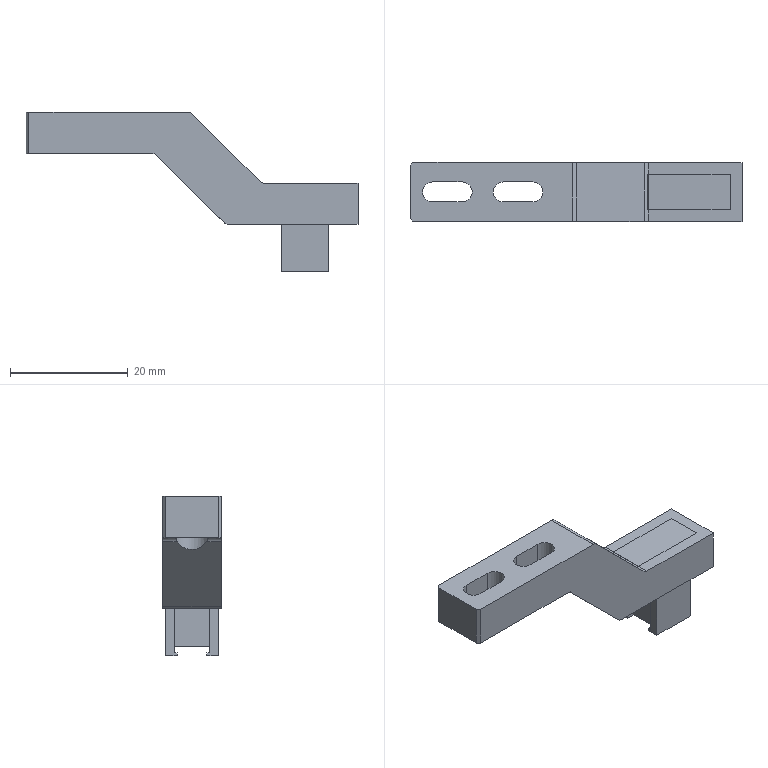NC program | NX | posted with a generic post | part box 56.3 x 10 x 27 mm
Lines 982 to 2462 of 3920, first 1366 of 1477 lines:
(ZLEVEL_PROFILE_COPY_2_COPY , TOOL : D4)
N1950 T04 M6
N1952 G54
N1954 G17 G0 G90 X-18.742 Y0.81 S9500 M3
N1956 G43 Z30. H4
N1958 Z-18.5
N1960 G94 G1 X-18.821 Y0.878 Z-18.505 F800.
N1962 X-19.178 Y1. Z-18.525
N1964 X-24.462 Z-18.802
N1966 X-24.792 Y0.893 Z-18.82
N1968 X-25.067 Y0.68 Z-18.839
N1970 X-25.253 Y0.387 Z-18.857
N1972 X-25.329 Y0.049 Z-18.875
N1974 X-25.286 Y-0.296 Z-18.893
N1976 X-25.166 Y-0.553 Z-18.908
N1978 X-24.977 Y-0.767 Z-18.923
N1980 X-24.736 Y-0.92 Z-18.938
N1982 X-24.462 Y-1. Z-18.953
N1984 X-19.178 Z-19.23
N1986 X-18.845 Y-0.891 Z-19.248
N1988 X-18.569 Y-0.675 Z-19.267
N1990 X-18.411 Y-0.439 Z-19.281
N1992 X-18.313 Y-0.074 Z-19.301
N1994 X-18.356 Y0.301 Z-19.321
N1996 X-18.534 Y0.634 Z-19.341
N1998 X-18.821 Y0.878 Z-19.361
N2000 X-19.178 Y1. Z-19.38
N2002 X-24.462 Z-19.657
N2004 X-24.792 Y0.893 Z-19.675
N2006 X-25.067 Y0.68 Z-19.694
N2008 X-25.253 Y0.387 Z-19.712
N2010 X-25.329 Y0.049 Z-19.73
N2012 X-25.286 Y-0.296 Z-19.748
N2014 X-25.166 Y-0.553 Z-19.763
N2016 X-24.977 Y-0.767 Z-19.778
N2018 X-24.736 Y-0.92 Z-19.793
N2020 X-24.462 Y-1. Z-19.808
N2022 X-19.178 Z-20.085
N2024 X-18.845 Y-0.891 Z-20.103
N2026 X-18.569 Y-0.675 Z-20.122
N2028 X-18.411 Y-0.439 Z-20.137
N2030 X-18.313 Y-0.074 Z-20.156
N2032 X-18.356 Y0.301 Z-20.176
N2034 X-18.534 Y0.634 Z-20.196
N2036 X-18.821 Y0.878 Z-20.216
N2038 X-19.178 Y1. Z-20.235
N2040 X-19.32 Z-20.243
N2042 X-24.32 F1100.
N2044 G3 X-25.32 Y0. R1.
N2046 X-24.32 Y-1. R1.
N2048 G1 X-19.32
N2050 G3 X-18.32 Y0. R1.
N2052 X-19.32 Y1. R1.
N2054 G1 X-19.459 Z-20.246
N2056 X-19.598 Y0.998 Z-20.248
N2058 X-19.737 Y1. Z-20.251
N2060 X-19.875 Y0.998 Z-20.254
N2062 X-20.014 Y1. Z-20.257
N2064 X-20.153 Y0.998 Z-20.259
N2066 X-20.292 Y1. Z-20.262
N2068 X-20.43 Y0.998 Z-20.265
N2070 X-20.569 Y1. Z-20.268
N2072 X-20.708 Y0.998 Z-20.27
N2074 X-20.847 Y1. Z-20.273
N2076 X-20.986 Y0.998 Z-20.276
N2078 X-21.124 Y1. Z-20.279
N2080 X-24.177 Z-20.339
N2082 X-24.316 Y0.994 Z-20.342
N2084 X-24.517 Y0.972 Z-20.346
N2086 X-24.588 Y0.955 Z-20.348
N2088 X-24.692 Y0.919 Z-20.35
N2090 X-24.776 Y0.883 Z-20.352
N2092 X-24.839 Y0.844 Z-20.353
N2094 X-24.987 Y0.733 Z-20.357
N2096 X-25.051 Y0.67 Z-20.359
N2098 X-25.152 Y0.539 Z-20.362
N2100 X-25.208 Y0.445 Z-20.364
N2102 X-25.248 Y0.349 Z-20.366
N2104 X-25.267 Y0.3 Z-20.367
N2106 X-25.276 Y0.261 Z-20.368
N2108 X-25.295 Y0.184 Z-20.37
N2110 X-25.308 Y0.079 Z-20.372
N2112 X-25.313 Y-0.013 Z-20.374
N2114 X-25.306 Y-0.089 Z-20.375
N2116 X-25.274 Y-0.267 Z-20.379
N2118 X-25.244 Y-0.356 Z-20.381
N2120 X-25.169 Y-0.51 Z-20.384
N2122 X-25.112 Y-0.597 Z-20.386
N2124 X-25.007 Y-0.716 Z-20.39
N2126 X-24.919 Y-0.791 Z-20.392
N2128 X-24.832 Y-0.848 Z-20.394
N2130 X-24.787 Y-0.875 Z-20.395
N2132 X-24.752 Y-0.893 Z-20.396
N2134 X-24.678 Y-0.923 Z-20.397
N2136 X-24.585 Y-0.954 Z-20.399
N2138 X-24.497 Y-0.975 Z-20.401
N2140 X-24.412 Y-0.985 Z-20.403
N2142 X-24.274 Y-1. Z-20.406
N2144 X-24.135 Z-20.408
N2146 X-20.249 Z-20.486
N2148 X-19.32
N2150 G3 X-18.32 Y0. R1.
N2152 X-19.32 Y1. R1.
N2154 G1 X-19.459 Z-20.488
N2156 X-19.598 Y0.998 Z-20.491
N2158 X-19.737 Y1. Z-20.494
N2160 X-19.875 Y0.998 Z-20.497
N2162 X-20.014 Y1. Z-20.5
N2164 X-20.153 Y0.998 Z-20.502
N2166 X-20.292 Y1. Z-20.505
N2168 X-20.43 Y0.998 Z-20.508
N2170 X-20.569 Y1. Z-20.511
N2172 X-20.708 Y0.998 Z-20.513
N2174 X-20.847 Y1. Z-20.516
N2176 X-20.986 Y0.998 Z-20.519
N2178 X-21.124 Y1. Z-20.522
N2180 X-24.177 Z-20.582
N2182 X-24.316 Y0.994 Z-20.585
N2184 X-24.517 Y0.972 Z-20.589
N2186 X-24.588 Y0.955 Z-20.591
N2188 X-24.692 Y0.919 Z-20.593
N2190 X-24.776 Y0.883 Z-20.595
N2192 X-24.839 Y0.844 Z-20.596
N2194 X-24.987 Y0.733 Z-20.6
N2196 X-25.051 Y0.67 Z-20.602
N2198 X-25.152 Y0.539 Z-20.605
N2200 X-25.208 Y0.445 Z-20.607
N2202 X-25.248 Y0.349 Z-20.609
N2204 X-25.267 Y0.3 Z-20.61
N2206 X-25.276 Y0.261 Z-20.611
N2208 X-25.294 Y0.184 Z-20.613
N2210 X-25.308 Y0.079 Z-20.615
N2212 X-25.313 Y-0.013 Z-20.617
N2214 X-25.306 Y-0.089 Z-20.618
N2216 X-25.274 Y-0.267 Z-20.622
N2218 X-25.244 Y-0.356 Z-20.624
N2220 X-25.169 Y-0.51 Z-20.627
N2222 X-25.112 Y-0.597 Z-20.629
N2224 X-25.007 Y-0.716 Z-20.632
N2226 X-24.919 Y-0.791 Z-20.635
N2228 X-24.832 Y-0.848 Z-20.637
N2230 X-24.787 Y-0.875 Z-20.638
N2232 X-24.752 Y-0.893 Z-20.639
N2234 X-24.678 Y-0.923 Z-20.64
N2236 X-24.585 Y-0.954 Z-20.642
N2238 X-24.497 Y-0.975 Z-20.644
N2240 X-24.412 Y-0.985 Z-20.646
N2242 X-24.274 Y-1. Z-20.649
N2244 X-24.135 Z-20.651
N2246 X-20.249 Z-20.729
N2248 X-19.32
N2250 G3 X-18.32 Y0. R1.
N2252 X-19.32 Y1. R1.
N2254 G1 X-19.459 Z-20.731
N2256 X-19.598 Y0.998 Z-20.734
N2258 X-19.737 Y1. Z-20.737
N2260 X-19.875 Y0.998 Z-20.74
N2262 X-20.014 Y1. Z-20.742
N2264 X-20.153 Y0.998 Z-20.745
N2266 X-20.292 Y1. Z-20.748
N2268 X-20.43 Y0.998 Z-20.751
N2270 X-20.569 Y1. Z-20.753
N2272 X-20.708 Y0.998 Z-20.756
N2274 X-20.847 Y1. Z-20.759
N2276 X-20.986 Y0.998 Z-20.762
N2278 X-21.124 Y1. Z-20.764
N2280 X-24.177 Z-20.825
N2282 X-24.316 Y0.994 Z-20.828
N2284 X-24.517 Y0.972 Z-20.832
N2286 X-24.588 Y0.955 Z-20.833
N2288 X-24.692 Y0.919 Z-20.836
N2290 X-24.776 Y0.883 Z-20.837
N2292 X-24.839 Y0.844 Z-20.839
N2294 X-24.986 Y0.733 Z-20.843
N2296 X-25.051 Y0.67 Z-20.844
N2298 X-25.151 Y0.54 Z-20.848
N2300 X-25.208 Y0.445 Z-20.85
N2302 X-25.248 Y0.349 Z-20.852
N2304 X-25.267 Y0.3 Z-20.853
N2306 X-25.276 Y0.262 Z-20.854
N2308 X-25.294 Y0.184 Z-20.856
N2310 X-25.308 Y0.079 Z-20.858
N2312 X-25.312 Y-0.013 Z-20.859
N2314 X-25.306 Y-0.089 Z-20.861
N2316 X-25.274 Y-0.266 Z-20.865
N2318 X-25.243 Y-0.356 Z-20.867
N2320 X-25.169 Y-0.51 Z-20.87
N2322 X-25.112 Y-0.597 Z-20.872
N2324 X-25.007 Y-0.716 Z-20.875
N2326 X-24.919 Y-0.791 Z-20.878
N2328 X-24.832 Y-0.848 Z-20.88
N2330 X-24.787 Y-0.875 Z-20.881
N2332 X-24.752 Y-0.892 Z-20.882
N2334 X-24.678 Y-0.923 Z-20.883
N2336 X-24.586 Y-0.954 Z-20.885
N2338 X-24.497 Y-0.975 Z-20.887
N2340 X-24.412 Y-0.985 Z-20.889
N2342 X-24.274 Y-1. Z-20.891
N2344 X-24.135 Z-20.894
N2346 X-20.249 Z-20.971
N2348 X-19.32
N2350 G3 X-18.32 Y0. R1.
N2352 X-19.32 Y1. R1.
N2354 G1 X-19.459 Z-20.974
N2356 X-19.598 Y0.998 Z-20.977
N2358 X-19.737 Y1. Z-20.98
N2360 X-19.875 Y0.998 Z-20.982
N2362 X-20.014 Y1. Z-20.985
N2364 X-20.153 Y0.998 Z-20.988
N2366 X-20.292 Y1. Z-20.991
N2368 X-20.43 Y0.998 Z-20.994
N2370 X-20.569 Y1. Z-20.996
N2372 X-20.708 Y0.998 Z-20.999
N2374 X-20.847 Y1. Z-21.002
N2376 X-20.986 Y0.998 Z-21.005
N2378 X-21.124 Y1. Z-21.007
N2380 X-24.177 Z-21.068
N2382 X-24.316 Y0.994 Z-21.071
N2384 X-24.517 Y0.972 Z-21.075
N2386 X-24.588 Y0.955 Z-21.076
N2388 X-24.692 Y0.919 Z-21.078
N2390 X-24.776 Y0.882 Z-21.08
N2392 X-24.839 Y0.844 Z-21.082
N2394 X-24.986 Y0.733 Z-21.086
N2396 X-25.051 Y0.67 Z-21.087
N2398 X-25.151 Y0.54 Z-21.091
N2400 X-25.208 Y0.445 Z-21.093
N2402 X-25.248 Y0.349 Z-21.095
N2404 X-25.266 Y0.3 Z-21.096
N2406 X-25.294 Y0.184 Z-21.098
N2408 X-25.308 Y0.079 Z-21.101
N2410 X-25.312 Y-0.012 Z-21.102
N2412 X-25.306 Y-0.089 Z-21.104
N2414 X-25.274 Y-0.266 Z-21.108
N2416 X-25.243 Y-0.356 Z-21.109
N2418 X-25.169 Y-0.509 Z-21.113
N2420 X-25.112 Y-0.597 Z-21.115
N2422 X-25.007 Y-0.715 Z-21.118
N2424 X-24.919 Y-0.791 Z-21.12
N2426 X-24.832 Y-0.848 Z-21.123
N2428 X-24.787 Y-0.874 Z-21.124
N2430 X-24.752 Y-0.892
N2432 X-24.678 Y-0.922 Z-21.126
N2434 X-24.586 Y-0.954 Z-21.128
N2436 X-24.497 Y-0.975 Z-21.13
N2438 X-24.412 Y-0.985 Z-21.131
N2440 X-24.274 Y-1. Z-21.134
N2442 X-24.135 Z-21.137
N2444 X-20.249 Z-21.214
N2446 X-19.32
N2448 G3 X-18.32 Y0. R1.
N2450 X-19.32 Y1. R1.
N2452 G1 X-19.459 Z-21.217
N2454 X-19.598 Y0.998 Z-21.22
N2456 X-19.737 Y1. Z-21.223
N2458 X-19.875 Y0.998 Z-21.225
N2460 X-20.014 Y1. Z-21.228
N2462 X-20.153 Y0.998 Z-21.231
N2464 X-20.292 Y1. Z-21.234
N2466 X-20.43 Y0.998 Z-21.236
N2468 X-20.569 Y1. Z-21.239
N2470 X-20.708 Y0.998 Z-21.242
N2472 X-20.847 Y1. Z-21.245
N2474 X-20.986 Y0.998 Z-21.247
N2476 X-21.124 Y1. Z-21.25
N2478 X-24.177 Z-21.311
N2480 X-24.316 Y0.994 Z-21.314
N2482 X-24.518 Y0.971 Z-21.318
N2484 X-24.588 Y0.955 Z-21.319
N2486 X-24.692 Y0.919 Z-21.321
N2488 X-24.776 Y0.882 Z-21.323
N2490 X-24.839 Y0.844 Z-21.325
N2492 X-24.986 Y0.733 Z-21.328
N2494 X-25.051 Y0.67 Z-21.33
N2496 X-25.151 Y0.54 Z-21.333
N2498 X-25.208 Y0.445 Z-21.336
N2500 X-25.248 Y0.349 Z-21.338
N2502 X-25.266 Y0.3 Z-21.339
N2504 X-25.294 Y0.184 Z-21.341
N2506 X-25.308 Y0.079 Z-21.343
N2508 X-25.312 Y-0.012 Z-21.345
N2510 X-25.306 Y-0.089 Z-21.347
N2512 X-25.274 Y-0.266 Z-21.35
N2514 X-25.243 Y-0.356 Z-21.352
N2516 X-25.169 Y-0.509 Z-21.356
N2518 X-25.112 Y-0.597 Z-21.358
N2520 X-25.007 Y-0.715 Z-21.361
N2522 X-24.919 Y-0.791 Z-21.363
N2524 X-24.832 Y-0.848 Z-21.365
N2526 X-24.787 Y-0.874 Z-21.366
N2528 X-24.752 Y-0.892 Z-21.367
N2530 X-24.678 Y-0.922 Z-21.369
N2532 X-24.586 Y-0.953 Z-21.371
N2534 X-24.497 Y-0.975 Z-21.373
N2536 X-24.412 Y-0.985 Z-21.374
N2538 X-24.274 Y-1. Z-21.377
N2540 X-24.135 Z-21.38
N2542 X-20.249 Z-21.457
N2544 X-19.32
N2546 G3 X-18.32 Y0. R1.
N2548 X-19.32 Y1. R1.
N2550 G1 X-19.459 Z-21.46
N2552 X-19.598 Y0.998 Z-21.463
N2554 X-19.737 Y1. Z-21.465
N2556 X-19.875 Y0.998 Z-21.468
N2558 X-20.014 Y1. Z-21.471
N2560 X-20.153 Y0.998 Z-21.474
N2562 X-20.292 Y1. Z-21.476
N2564 X-20.43 Y0.998 Z-21.479
N2566 X-20.569 Y1. Z-21.482
N2568 X-20.708 Y0.998 Z-21.485
N2570 X-20.847 Y1. Z-21.488
N2572 X-20.986 Y0.998 Z-21.49
N2574 X-21.124 Y1. Z-21.493
N2576 X-24.177 Z-21.554
N2578 X-24.316 Y0.994 Z-21.556
N2580 X-24.518 Y0.971 Z-21.561
N2582 X-24.588 Y0.955 Z-21.562
N2584 X-24.691 Y0.919 Z-21.564
N2586 X-24.775 Y0.882 Z-21.566
N2588 X-24.839 Y0.844 Z-21.568
N2590 X-24.986 Y0.733 Z-21.571
N2592 X-25.051 Y0.67 Z-21.573
N2594 X-25.151 Y0.54 Z-21.576
N2596 X-25.208 Y0.445 Z-21.579
N2598 X-25.248 Y0.349 Z-21.581
N2600 X-25.266 Y0.3 Z-21.582
N2602 X-25.294 Y0.184 Z-21.584
N2604 X-25.308 Y0.079 Z-21.586
N2606 X-25.312 Y-0.012 Z-21.588
N2608 X-25.306 Y-0.089 Z-21.59
N2610 X-25.274 Y-0.266 Z-21.593
N2612 X-25.243 Y-0.356 Z-21.595
N2614 X-25.169 Y-0.509 Z-21.599
N2616 X-25.112 Y-0.597 Z-21.601
N2618 X-25.007 Y-0.715 Z-21.604
N2620 X-24.918 Y-0.791 Z-21.606
N2622 X-24.832 Y-0.847 Z-21.608
N2624 X-24.787 Y-0.874 Z-21.609
N2626 X-24.752 Y-0.892 Z-21.61
N2628 X-24.678 Y-0.922 Z-21.612
N2630 X-24.586 Y-0.953 Z-21.614
N2632 X-24.497 Y-0.975 Z-21.615
N2634 X-24.412 Y-0.985 Z-21.617
N2636 X-24.274 Y-1. Z-21.62
N2638 X-24.135 Z-21.623
N2640 X-20.249 Z-21.7
N2642 X-19.32
N2644 G3 X-18.32 Y0. R1.
N2646 X-19.32 Y1. R1.
N2648 G1 X-19.459 Z-21.703
N2650 X-19.598 Y0.998 Z-21.706
N2652 X-19.737 Y1. Z-21.708
N2654 X-19.875 Y0.998 Z-21.711
N2656 X-20.014 Y1. Z-21.714
N2658 X-20.153 Y0.998 Z-21.717
N2660 X-20.292 Y1. Z-21.719
N2662 X-20.43 Y0.998 Z-21.722
N2664 X-20.569 Y1. Z-21.725
N2666 X-20.708 Y0.998 Z-21.728
N2668 X-20.847 Y1. Z-21.73
N2670 X-20.986 Y0.998 Z-21.733
N2672 X-21.124 Y1. Z-21.736
N2674 X-24.177 Z-21.797
N2676 X-24.316 Y0.994 Z-21.799
N2678 X-24.518 Y0.971 Z-21.803
N2680 X-24.588 Y0.955 Z-21.805
N2682 X-24.691 Y0.919 Z-21.807
N2684 X-24.775 Y0.882 Z-21.809
N2686 X-24.839 Y0.844 Z-21.81
N2688 X-24.986 Y0.734 Z-21.814
N2690 X-25.051 Y0.67 Z-21.816
N2692 X-25.153 Y0.537 Z-21.819
N2694 X-25.208 Y0.445 Z-21.821
N2696 X-25.248 Y0.348 Z-21.824
N2698 X-25.266 Y0.3 Z-21.825
N2700 X-25.294 Y0.184 Z-21.827
N2702 X-25.308 Y0.079 Z-21.829
N2704 X-25.313 Y-0.012 Z-21.831
N2706 X-25.306 Y-0.089 Z-21.832
N2708 X-25.272 Y-0.272 Z-21.836
N2710 X-25.243 Y-0.356 Z-21.838
N2712 X-25.168 Y-0.511 Z-21.841
N2714 X-25.112 Y-0.597 Z-21.844
N2716 X-25.007 Y-0.715 Z-21.847
N2718 X-24.918 Y-0.791 Z-21.849
N2720 X-24.832 Y-0.847 Z-21.851
N2722 X-24.787 Y-0.874 Z-21.852
N2724 X-24.752 Y-0.892 Z-21.853
N2726 X-24.678 Y-0.922 Z-21.855
N2728 X-24.586 Y-0.953 Z-21.856
N2730 X-24.497 Y-0.975 Z-21.858
N2732 X-24.412 Y-0.985 Z-21.86
N2734 X-24.274 Y-1. Z-21.863
N2736 X-24.135 Z-21.866
N2738 X-20.249 Z-21.943
N2740 X-19.32
N2742 G3 X-18.32 Y0. R1.
N2744 X-19.32 Y1. R1.
N2746 G1 X-19.459 Z-21.946
N2748 X-19.598 Y0.998 Z-21.948
N2750 X-19.737 Y1. Z-21.951
N2752 X-19.875 Y0.998 Z-21.954
N2754 X-20.014 Y1. Z-21.957
N2756 X-20.153 Y0.998 Z-21.959
N2758 X-20.292 Y1. Z-21.962
N2760 X-20.43 Y0.998 Z-21.965
N2762 X-20.569 Y1. Z-21.968
N2764 X-20.708 Y0.998 Z-21.97
N2766 X-20.847 Y1. Z-21.973
N2768 X-20.986 Y0.998 Z-21.976
N2770 X-21.124 Y1. Z-21.979
N2772 X-24.177 Z-22.039
N2774 X-24.316 Y0.994 Z-22.042
N2776 X-24.518 Y0.971 Z-22.046
N2778 X-24.588 Y0.954 Z-22.048
N2780 X-24.691 Y0.919 Z-22.05
N2782 X-24.775 Y0.882 Z-22.052
N2784 X-24.839 Y0.844 Z-22.053
N2786 X-24.986 Y0.734 Z-22.057
N2788 X-25.051 Y0.67 Z-22.059
N2790 X-25.153 Y0.537 Z-22.062
N2792 X-25.207 Y0.445 Z-22.064
N2794 X-25.248 Y0.348 Z-22.066
N2796 X-25.266 Y0.3 Z-22.067
N2798 X-25.294 Y0.184 Z-22.07
N2800 X-25.307 Y0.079 Z-22.072
N2802 X-25.313 Y-0.012 Z-22.074
N2804 X-25.306 Y-0.089 Z-22.075
N2806 X-25.272 Y-0.271 Z-22.079
N2808 X-25.243 Y-0.356 Z-22.081
N2810 X-25.168 Y-0.511 Z-22.084
N2812 X-25.112 Y-0.597 Z-22.086
N2814 X-25.007 Y-0.715 Z-22.09
N2816 X-24.918 Y-0.791 Z-22.092
N2818 X-24.832 Y-0.847 Z-22.094
N2820 X-24.787 Y-0.874 Z-22.095
N2822 X-24.752 Y-0.892 Z-22.096
N2824 X-24.678 Y-0.922 Z-22.097
N2826 X-24.587 Y-0.954 Z-22.099
N2828 X-24.498 Y-0.975 Z-22.101
N2830 X-24.412 Y-0.985 Z-22.103
N2832 X-24.274 Y-1. Z-22.106
N2834 X-24.135 Z-22.108
N2836 X-20.249 Z-22.186
N2838 X-19.32
N2840 G3 X-18.32 Y0. R1.
N2842 X-19.32 Y1. R1.
N2844 G1 X-19.459 Z-22.188
N2846 X-19.598 Y0.998 Z-22.191
N2848 X-19.737 Y1. Z-22.194
N2850 X-19.875 Y0.998 Z-22.197
N2852 X-20.014 Y1. Z-22.2
N2854 X-20.153 Y0.998 Z-22.202
N2856 X-20.292 Y1. Z-22.205
N2858 X-20.43 Y0.998 Z-22.208
N2860 X-20.569 Y1. Z-22.211
N2862 X-20.708 Y0.998 Z-22.213
N2864 X-20.847 Y1. Z-22.216
N2866 X-20.986 Y0.998 Z-22.219
N2868 X-21.124 Y1. Z-22.222
N2870 X-24.177 Z-22.282
N2872 X-24.316 Y0.994 Z-22.285
N2874 X-24.518 Y0.971 Z-22.289
N2876 X-24.588 Y0.954 Z-22.291
N2878 X-24.691 Y0.919 Z-22.293
N2880 X-24.775 Y0.882 Z-22.295
N2882 X-24.839 Y0.844 Z-22.296
N2884 X-24.986 Y0.735 Z-22.3
N2886 X-25.051 Y0.67 Z-22.302
N2888 X-25.153 Y0.537 Z-22.305
N2890 X-25.207 Y0.445 Z-22.307
N2892 X-25.248 Y0.349 Z-22.309
N2894 X-25.266 Y0.3 Z-22.31
N2896 X-25.294 Y0.184 Z-22.313
N2898 X-25.307 Y0.079 Z-22.315
N2900 X-25.313 Y-0.012 Z-22.317
N2902 X-25.306 Y-0.089 Z-22.318
N2904 X-25.272 Y-0.271 Z-22.322
N2906 X-25.243 Y-0.356 Z-22.324
N2908 X-25.168 Y-0.51 Z-22.327
N2910 X-25.112 Y-0.597 Z-22.329
N2912 X-25.007 Y-0.715 Z-22.332
N2914 X-24.918 Y-0.791 Z-22.335
N2916 X-24.832 Y-0.847 Z-22.337
N2918 X-24.788 Y-0.874 Z-22.338
N2920 X-24.752 Y-0.892 Z-22.339
N2922 X-24.678 Y-0.922 Z-22.34
N2924 X-24.587 Y-0.954 Z-22.342
N2926 X-24.498 Y-0.975 Z-22.344
N2928 X-24.412 Y-0.985 Z-22.346
N2930 X-24.274 Y-1. Z-22.349
N2932 X-24.135 Z-22.351
N2934 X-20.249 Z-22.429
N2936 X-19.32
N2938 G3 X-18.32 Y0. R1.
N2940 X-19.32 Y1. R1.
N2942 G1 X-19.459 Z-22.431
N2944 X-19.598 Y0.998 Z-22.434
N2946 X-19.737 Y1. Z-22.437
N2948 X-19.875 Y0.998 Z-22.44
N2950 X-20.014 Y1. Z-22.442
N2952 X-20.153 Y0.998 Z-22.445
N2954 X-20.292 Y1. Z-22.448
N2956 X-20.43 Y0.998 Z-22.451
N2958 X-20.569 Y1. Z-22.453
N2960 X-20.708 Y0.998 Z-22.456
N2962 X-20.847 Y1. Z-22.459
N2964 X-20.986 Y0.998 Z-22.462
N2966 X-21.124 Y1. Z-22.464
N2968 X-24.177 Z-22.525
N2970 X-24.316 Y0.994 Z-22.528
N2972 X-24.518 Y0.971 Z-22.532
N2974 X-24.588 Y0.954 Z-22.533
N2976 X-24.691 Y0.918 Z-22.536
N2978 X-24.775 Y0.882 Z-22.537
N2980 X-24.839 Y0.844 Z-22.539
N2982 X-24.986 Y0.735 Z-22.543
N2984 X-25.051 Y0.67 Z-22.544
N2986 X-25.153 Y0.537 Z-22.548
N2988 X-25.207 Y0.445 Z-22.55
N2990 X-25.248 Y0.349 Z-22.552
N2992 X-25.267 Y0.3 Z-22.553
N2994 X-25.294 Y0.184 Z-22.556
N2996 X-25.307 Y0.077 Z-22.558
N2998 X-25.312 Y-0.014 Z-22.56
N3000 X-25.305 Y-0.089 Z-22.561
N3002 X-25.273 Y-0.266 Z-22.565
N3004 X-25.243 Y-0.356 Z-22.567
N3006 X-25.169 Y-0.509 Z-22.57
N3008 X-25.112 Y-0.597 Z-22.572
N3010 X-25.007 Y-0.715 Z-22.575
N3012 X-24.918 Y-0.791 Z-22.578
N3014 X-24.832 Y-0.847 Z-22.58
N3016 X-24.788 Y-0.874 Z-22.581
N3018 X-24.752 Y-0.892 Z-22.582
N3020 X-24.678 Y-0.922 Z-22.583
N3022 X-24.587 Y-0.954 Z-22.585
N3024 X-24.498 Y-0.975 Z-22.587
N3026 X-24.412 Y-0.985 Z-22.589
N3028 X-24.274 Y-1. Z-22.591
N3030 X-24.135 Z-22.594
N3032 X-20.249 Z-22.671
N3034 X-19.32
N3036 G3 X-18.32 Y0. R1.
N3038 X-19.32 Y1. R1.
N3040 G1 X-19.459 Z-22.674
N3042 X-19.598 Y0.998 Z-22.677
N3044 X-19.737 Y1. Z-22.68
N3046 X-19.875 Y0.998 Z-22.682
N3048 X-20.014 Y1. Z-22.685
N3050 X-20.153 Y0.998 Z-22.688
N3052 X-20.292 Y1. Z-22.691
N3054 X-20.43 Y0.998 Z-22.694
N3056 X-20.569 Y1. Z-22.696
N3058 X-20.708 Y0.998 Z-22.699
N3060 X-20.847 Y1. Z-22.702
N3062 X-20.986 Y0.998 Z-22.705
N3064 X-21.124 Y1. Z-22.707
N3066 X-24.177 Z-22.768
N3068 X-24.316 Y0.993 Z-22.771
N3070 X-24.518 Y0.971 Z-22.775
N3072 X-24.588 Y0.954 Z-22.776
N3074 X-24.691 Y0.918 Z-22.778
N3076 X-24.775 Y0.882 Z-22.78
N3078 X-24.839 Y0.844 Z-22.782
N3080 X-24.985 Y0.735 Z-22.785
N3082 X-25.051 Y0.67 Z-22.787
N3084 X-25.152 Y0.537 Z-22.791
N3086 X-25.207 Y0.445 Z-22.793
N3088 X-25.248 Y0.349 Z-22.795
N3090 X-25.267 Y0.3 Z-22.796
N3092 X-25.276 Y0.262 Z-22.797
N3094 X-25.294 Y0.184 Z-22.798
N3096 X-25.307 Y0.076 Z-22.801
N3098 X-25.312 Y-0.015 Z-22.802
N3100 X-25.305 Y-0.089 Z-22.804
N3102 X-25.273 Y-0.267 Z-22.808
N3104 X-25.243 Y-0.356 Z-22.809
N3106 X-25.169 Y-0.509 Z-22.813
N3108 X-25.112 Y-0.597 Z-22.815
N3110 X-25.007 Y-0.715 Z-22.818
N3112 X-24.918 Y-0.791 Z-22.82
N3114 X-24.832 Y-0.847 Z-22.823
N3116 X-24.788 Y-0.874 Z-22.824
N3118 X-24.752 Y-0.892
N3120 X-24.678 Y-0.922 Z-22.826
N3122 X-24.587 Y-0.954 Z-22.828
N3124 X-24.498 Y-0.974 Z-22.83
N3126 X-24.412 Y-0.985 Z-22.831
N3128 X-24.274 Y-1. Z-22.834
N3130 X-24.135 Z-22.837
N3132 X-20.249 Z-22.914
N3134 X-19.32
N3136 G3 X-18.32 Y0. R1.
N3138 X-19.32 Y1. R1.
N3140 G1 X-24.233 Z-23.012
N3142 X-24.374 Y0.999 Z-23.015
N3144 X-24.513 Y0.981 Z-23.018
N3146 X-24.648 Y0.945 Z-23.02
N3148 X-24.777 Y0.89 Z-23.023
N3150 X-24.897 Y0.817 Z-23.026
N3152 X-25.006 Y0.728 Z-23.029
N3154 X-25.101 Y0.625 Z-23.032
N3156 X-25.181 Y0.51 Z-23.034
N3158 X-25.243 Y0.384 Z-23.037
N3160 X-25.288 Y0.251 Z-23.04
N3162 X-25.314 Y0.113 Z-23.043
N3164 X-25.32 Y-0.027 Z-23.045
N3166 X-25.306 Y-0.166 Z-23.048
N3168 X-25.273 Y-0.303 Z-23.051
N3170 X-25.222 Y-0.433 Z-23.054
N3172 X-25.152 Y-0.555 Z-23.057
N3174 X-25.066 Y-0.666 Z-23.059
N3176 X-24.966 Y-0.764 Z-23.062
N3178 X-24.853 Y-0.846 Z-23.065
N3180 X-24.729 Y-0.913 Z-23.068
N3182 X-24.597 Y-0.961 Z-23.071
N3184 X-24.46 Y-0.99 Z-23.073
N3186 X-24.32 Y-1. Z-23.076
N3188 X-20.249 Z-23.157
N3190 X-19.32
N3192 G3 X-18.32 Y0. R1.
N3194 X-19.32 Y1. R1.
N3196 G1 X-24.233 Z-23.255
N3198 X-24.374 Y0.999 Z-23.258
N3200 X-24.513 Y0.981 Z-23.26
N3202 X-24.648 Y0.945 Z-23.263
N3204 X-24.777 Y0.89 Z-23.266
N3206 X-24.897 Y0.817 Z-23.269
N3208 X-25.006 Y0.728 Z-23.272
N3210 X-25.101 Y0.625 Z-23.274
N3212 X-25.181 Y0.51 Z-23.277
N3214 X-25.243 Y0.384 Z-23.28
N3216 X-25.288 Y0.251 Z-23.283
N3218 X-25.314 Y0.113 Z-23.286
N3220 X-25.32 Y-0.027 Z-23.288
N3222 X-25.306 Y-0.166 Z-23.291
N3224 X-25.273 Y-0.303 Z-23.294
N3226 X-25.222 Y-0.433 Z-23.297
N3228 X-25.152 Y-0.555 Z-23.3
N3230 X-25.066 Y-0.666 Z-23.302
N3232 X-24.966 Y-0.764 Z-23.305
N3234 X-24.853 Y-0.846 Z-23.308
N3236 X-24.729 Y-0.913 Z-23.311
N3238 X-24.597 Y-0.961 Z-23.313
N3240 X-24.46 Y-0.99 Z-23.316
N3242 X-24.32 Y-1. Z-23.319
N3244 X-20.249 Z-23.4
N3246 X-19.32
N3248 G3 X-18.32 Y0. R1.
N3250 X-19.32 Y1. R1.
N3252 G1 X-24.32
N3254 G3 X-25.32 Y0. R1.
N3256 X-24.32 Y-1. R1.
N3258 G1 X-20.249
N3260 Z-21.9
N3262 G0 Z30.
N3264 X-6.378 Y0.342
N3266 Z-18.5
N3268 G1 X-6.393 Y0.4 Z-18.503 F800.
N3270 X-6.562 Y0.667 Z-18.52
N3272 X-6.669 Y0.759 Z-18.527
N3274 X-6.688 Y0.746 Z-18.528
N3276 X-7.155 Y0.891 Z-18.554
N3278 X-7.406 Y1. Z-18.568
N3280 X-12.462 Z-18.833
N3282 X-12.792 Y0.893 Z-18.851
N3284 X-13.067 Y0.68 Z-18.87
N3286 X-13.253 Y0.387 Z-18.888
N3288 X-13.329 Y0.048 Z-18.906
N3290 X-13.286 Y-0.296 Z-18.924
N3292 X-13.166 Y-0.553 Z-18.939
N3294 X-12.977 Y-0.767 Z-18.954
N3296 X-12.736 Y-0.92 Z-18.969
N3298 X-12.462 Y-1. Z-18.984
N3300 X-7.178 Z-19.261
N3302 X-6.806 Y-0.87 Z-19.282
N3304 X-6.513 Y-0.607 Z-19.302
N3306 X-6.444 Y-0.482 Z-19.31
N3308 X-6.467 Y-0.464 Z-19.311
N3310 X-6.463 Y-0.434 Z-19.313
N3312 X-6.437 Y-0.422 Z-19.314
N3314 X-6.443 Y-0.386 Z-19.316
N3316 X-6.42 Y-0.356 Z-19.318
N3318 X-6.384 Y-0.353 Z-19.32
N3320 X-6.334 Y-0.22 Z-19.327
N3322 X-6.315 Y0.095 Z-19.344
N3324 X-6.393 Y0.4 Z-19.36
N3326 X-6.562 Y0.667 Z-19.377
N3328 X-6.669 Y0.759 Z-19.384
N3330 X-6.688 Y0.746 Z-19.386
N3332 X-7.155 Y0.891 Z-19.411
N3334 X-7.406 Y1. Z-19.426
N3336 X-12.462 Z-19.691
N3338 X-12.792 Y0.893 Z-19.709
N3340 X-13.067 Y0.68 Z-19.727
N3342 X-13.253 Y0.387 Z-19.745
N3344 X-13.329 Y0.048 Z-19.763
N3346 X-13.286 Y-0.296 Z-19.781
N3348 X-13.166 Y-0.553 Z-19.796
N3350 X-12.977 Y-0.767 Z-19.811
N3352 X-12.736 Y-0.92 Z-19.826
N3354 X-12.462 Y-1. Z-19.841
N3356 X-7.178 Z-20.118
N3358 X-6.806 Y-0.87 Z-20.139
N3360 X-6.513 Y-0.607 Z-20.159
N3362 X-6.444 Y-0.482 Z-20.167
N3364 X-6.467 Y-0.464 Z-20.168
N3366 X-6.463 Y-0.434 Z-20.17
N3368 X-6.437 Y-0.422 Z-20.171
N3370 X-6.443 Y-0.386 Z-20.173
N3372 X-6.42 Y-0.356 Z-20.175
N3374 X-6.384 Y-0.353 Z-20.177
N3376 X-6.334 Y-0.22 Z-20.185
N3378 X-6.315 Y0.095 Z-20.201
N3380 X-6.393 Y0.4 Z-20.218
N3382 X-6.562 Y0.667 Z-20.234
N3384 X-6.669 Y0.759 Z-20.242
N3386 X-6.688 Y0.746 Z-20.243
N3388 X-7.155 Y0.891 F1100.
N3390 X-7.406 Y1.
N3392 X-12.32
N3394 G3 X-13.32 Y0. R1.
N3396 X-12.32 Y-1. R1.
N3398 G1 X-7.32
N3400 G3 X-6.444 Y-0.482 R1.
N3402 G1 X-6.467 Y-0.464
N3404 X-6.463 Y-0.434
N3406 X-6.437 Y-0.422
N3408 X-6.443 Y-0.386
N3410 X-6.42 Y-0.356
N3412 X-6.384 Y-0.353
N3414 G3 X-6.669 Y0.759 R1.
N3416 G1 X-6.688 Y0.746
N3418 X-6.821 Y0.788 Z-20.246
N3420 X-6.953 Y0.829 Z-20.248
N3422 X-7.086 Y0.87 Z-20.251
N3424 X-7.218 Y0.914 Z-20.254
N3426 X-7.282 Y0.939 Z-20.255
N3428 X-7.345 Y0.967 Z-20.257
N3430 X-7.377 Y0.981
N3432 X-7.408 Y0.996 Z-20.258
N3434 X-7.443 Y0.998 Z-20.259
N3436 X-7.477
N3438 X-7.616 Y1. Z-20.262
N3440 X-7.755 Y0.999 Z-20.265
N3442 X-7.894 Y0.998 Z-20.268
N3444 X-8.033 Z-20.27
N3446 X-8.172 Z-20.273
N3448 X-8.311 Z-20.276
N3450 X-8.449 Z-20.279
N3452 X-8.588 Z-20.281
N3454 X-8.727 Z-20.284
N3456 X-8.866 Z-20.287
N3458 X-9.005 Y1. Z-20.29
N3460 X-12.201 Z-20.353
N3462 X-12.339 Y0.992 Z-20.356
N3464 X-12.477 Y0.981 Z-20.359
N3466 X-12.574 Y0.958 Z-20.361
N3468 X-12.623 Y0.946 Z-20.362
N3470 X-12.662 Y0.93 Z-20.363
N3472 X-12.739 Y0.899 Z-20.364
N3474 X-12.834 Y0.848 Z-20.366
N3476 X-12.911 Y0.799 Z-20.368
N3478 X-12.969 Y0.749 Z-20.37
N3480 X-13.096 Y0.617 Z-20.373
N3482 X-13.15 Y0.543 Z-20.375
N3484 X-13.23 Y0.393 Z-20.379
N3486 X-13.268 Y0.295 Z-20.381
N3488 X-13.292 Y0.194 Z-20.383
N3490 X-13.302 Y0.143 Z-20.384
N3492 X-13.306 Y0.103 Z-20.385
N3494 X-13.311 Y0.023 Z-20.386
N3496 X-13.307 Y-0.088 Z-20.389
N3498 X-13.302 Y-0.144 Z-20.39
N3500 X-13.295 Y-0.179
N3502 X-13.278 Y-0.249 Z-20.392
N3504 X-13.218 Y-0.417 Z-20.395
N3506 X-13.173 Y-0.502 Z-20.397
N3508 X-13.076 Y-0.638 Z-20.401
N3510 X-13.003 Y-0.718 Z-20.403
N3512 X-12.878 Y-0.819 Z-20.406
N3514 X-12.781 Y-0.878 Z-20.408
N3516 X-12.647 Y-0.936 Z-20.411
N3518 X-12.522 Y-0.97 Z-20.414
N3520 X-12.385 Y-0.988 Z-20.417
N3522 X-12.247 Y-1. Z-20.419
N3524 X-8.913 Z-20.486
N3526 X-7.32
N3528 G3 X-6.444 Y-0.482 R1.
N3530 G1 X-6.467 Y-0.464
N3532 X-6.463 Y-0.434
N3534 X-6.437 Y-0.422
N3536 X-6.443 Y-0.386
N3538 X-6.42 Y-0.356
N3540 X-6.384 Y-0.353
N3542 G3 X-6.669 Y0.759 R1.
N3544 G1 X-6.688 Y0.746
N3546 X-6.821 Y0.788 Z-20.488
N3548 X-6.953 Y0.829 Z-20.491
N3550 X-7.086 Y0.87 Z-20.494
N3552 X-7.218 Y0.914 Z-20.497
N3554 X-7.282 Y0.939 Z-20.498
N3556 X-7.345 Y0.967 Z-20.5
N3558 X-7.377 Y0.982
N3560 X-7.408 Y0.995 Z-20.501
N3562 X-7.443 Y0.998 Z-20.502
N3564 X-7.477
N3566 X-7.616 Y1. Z-20.505
N3568 X-7.755 Y0.999 Z-20.508
N3570 X-7.894 Y0.998 Z-20.511
N3572 X-8.033 Z-20.513
N3574 X-8.172 Z-20.516
N3576 X-8.311 Z-20.519
N3578 X-8.449 Z-20.522
N3580 X-8.588 Z-20.524
N3582 X-8.727 Z-20.527
N3584 X-8.866 Z-20.53
N3586 X-9.005 Y1. Z-20.533
N3588 X-12.201 Z-20.596
N3590 X-12.339 Y0.992 Z-20.599
N3592 X-12.477 Y0.981 Z-20.602
N3594 X-12.574 Y0.958 Z-20.604
N3596 X-12.623 Y0.946 Z-20.605
N3598 X-12.662 Y0.93
N3600 X-12.739 Y0.899 Z-20.607
N3602 X-12.833 Y0.848 Z-20.609
N3604 X-12.911 Y0.799 Z-20.611
N3606 X-12.969 Y0.749 Z-20.613
N3608 X-13.096 Y0.617 Z-20.616
N3610 X-13.15 Y0.543 Z-20.618
N3612 X-13.23 Y0.393 Z-20.622
N3614 X-13.268 Y0.295 Z-20.624
N3616 X-13.292 Y0.194 Z-20.626
N3618 X-13.302 Y0.144 Z-20.627
N3620 X-13.306 Y0.104 Z-20.628
N3622 X-13.311 Y0.023 Z-20.629
N3624 X-13.307 Y-0.088 Z-20.631
N3626 X-13.302 Y-0.144 Z-20.633
N3628 X-13.295 Y-0.179
N3630 X-13.278 Y-0.249 Z-20.635
N3632 X-13.218 Y-0.417 Z-20.638
N3634 X-13.173 Y-0.502 Z-20.64
N3636 X-13.076 Y-0.638 Z-20.644
N3638 X-13.003 Y-0.718 Z-20.646
N3640 X-12.878 Y-0.819 Z-20.649
N3642 X-12.781 Y-0.878 Z-20.651
N3644 X-12.647 Y-0.936 Z-20.654
N3646 X-12.522 Y-0.97 Z-20.657
N3648 X-12.385 Y-0.988 Z-20.66
N3650 X-12.247 Y-1. Z-20.662
N3652 X-8.913 Z-20.729
N3654 X-7.32
N3656 G3 X-6.444 Y-0.482 R1.
N3658 G1 X-6.467 Y-0.464
N3660 X-6.463 Y-0.434
N3662 X-6.437 Y-0.422
N3664 X-6.443 Y-0.386
N3666 X-6.42 Y-0.356
N3668 X-6.384 Y-0.353
N3670 G3 X-6.669 Y0.759 R1.
N3672 G1 X-6.688 Y0.746
N3674 X-6.821 Y0.788 Z-20.731
N3676 X-6.953 Y0.829 Z-20.734
N3678 X-7.086 Y0.87 Z-20.737
N3680 X-7.218 Y0.914 Z-20.74
N3682 X-7.282 Y0.939 Z-20.741
N3684 X-7.345 Y0.967 Z-20.742
N3686 X-7.377 Y0.981 Z-20.743
N3688 X-7.408 Y0.996 Z-20.744
N3690 X-7.443 Y0.997
N3692 X-7.477 Y0.998 Z-20.745
N3694 X-7.616 Y1. Z-20.748
N3696 X-7.755 Y0.998 Z-20.751
N3698 X-7.894 Z-20.753
N3700 X-8.033 Z-20.756
N3702 X-8.172 Z-20.759
N3704 X-8.311 Z-20.762
N3706 X-8.449 Z-20.764
N3708 X-8.588 Z-20.767
N3710 X-8.727 Z-20.77
N3712 X-8.866 Z-20.773
N3714 X-9.005 Y1. Z-20.775
N3716 X-12.201 Z-20.839
N3718 X-12.339 Y0.992 Z-20.842
N3720 X-12.477 Y0.981 Z-20.844
N3722 X-12.574 Y0.958 Z-20.846
N3724 X-12.623 Y0.946 Z-20.847
N3726 X-12.662 Y0.93 Z-20.848
N3728 X-12.739 Y0.899 Z-20.85
N3730 X-12.833 Y0.848 Z-20.852
N3732 X-12.91 Y0.799 Z-20.854
N3734 X-12.969 Y0.749 Z-20.856
N3736 X-13.096 Y0.617 Z-20.859
N3738 X-13.15 Y0.543 Z-20.861
N3740 X-13.23 Y0.393 Z-20.864
N3742 X-13.268 Y0.294 Z-20.867
N3744 X-13.292 Y0.194 Z-20.869
N3746 X-13.303 Y0.144 Z-20.87
N3748 X-13.306 Y0.104
N3750 X-13.311 Y0.023 Z-20.872
N3752 X-13.306 Y-0.088 Z-20.874
N3754 X-13.302 Y-0.144 Z-20.875
N3756 X-13.295 Y-0.179 Z-20.876
N3758 X-13.278 Y-0.249 Z-20.878
N3760 X-13.241 Y-0.362 Z-20.88
N3762 X-13.207 Y-0.447 Z-20.882
N3764 X-13.173 Y-0.502 Z-20.883
N3766 X-13.061 Y-0.657 Z-20.887
N3768 X-13.003 Y-0.718 Z-20.889
N3770 X-12.872 Y-0.822 Z-20.892
N3772 X-12.781 Y-0.878 Z-20.894
N3774 X-12.648 Y-0.935 Z-20.897
N3776 X-12.522 Y-0.97 Z-20.9
N3778 X-12.385 Y-0.988 Z-20.902
N3780 X-12.247 Y-1. Z-20.905
N3782 X-8.913 Z-20.971
N3784 X-7.32
N3786 G3 X-6.444 Y-0.482 R1.
N3788 G1 X-6.467 Y-0.464
N3790 X-6.463 Y-0.434
N3792 X-6.437 Y-0.422
N3794 X-6.443 Y-0.386
N3796 X-6.42 Y-0.356
N3798 X-6.384 Y-0.353
N3800 G3 X-6.669 Y0.759 R1.
N3802 G1 X-6.688 Y0.746
N3804 X-6.821 Y0.788 Z-20.974
N3806 X-6.953 Y0.829 Z-20.977
N3808 X-7.086 Y0.87 Z-20.98
N3810 X-7.218 Y0.914 Z-20.982
N3812 X-7.282 Y0.939 Z-20.984
N3814 X-7.345 Y0.967 Z-20.985
N3816 X-7.377 Y0.981 Z-20.986
N3818 X-7.408 Y0.996 Z-20.987
N3820 X-7.443 Y0.997
N3822 X-7.477 Y0.998 Z-20.988
N3824 X-7.616 Y1. Z-20.991
N3826 X-7.755 Y0.998 Z-20.994
N3828 X-7.894 Z-20.996
N3830 X-8.033 Z-20.999
N3832 X-8.172 Z-21.002
N3834 X-8.311 Z-21.005
N3836 X-8.449 Z-21.007
N3838 X-8.588 Z-21.01
N3840 X-8.727 Z-21.013
N3842 X-8.866 Z-21.016
N3844 X-9.005 Y1. Z-21.018
N3846 X-12.201 Z-21.082
N3848 X-12.339 Y0.992 Z-21.085
N3850 X-12.477 Y0.981 Z-21.087
N3852 X-12.574 Y0.958 Z-21.089
N3854 X-12.623 Y0.946 Z-21.09
N3856 X-12.739 Y0.899 Z-21.093
N3858 X-12.833 Y0.848 Z-21.095
N3860 X-12.91 Y0.799 Z-21.097
N3862 X-12.969 Y0.749 Z-21.098
N3864 X-13.096 Y0.618 Z-21.102
N3866 X-13.15 Y0.543 Z-21.104
N3868 X-13.23 Y0.394 Z-21.107
N3870 X-13.268 Y0.294 Z-21.109
N3872 X-13.292 Y0.194 Z-21.111
N3874 X-13.303 Y0.144 Z-21.113
N3876 X-13.306 Y0.104
N3878 X-13.311 Y0.023 Z-21.115
N3880 X-13.306 Y-0.088 Z-21.117
N3882 X-13.302 Y-0.143 Z-21.118
N3884 X-13.295 Y-0.179 Z-21.119
N3886 X-13.278 Y-0.249 Z-21.12
N3888 X-13.242 Y-0.362 Z-21.123
N3890 X-13.207 Y-0.446 Z-21.125
N3892 X-13.173 Y-0.502 Z-21.126
N3894 X-13.061 Y-0.657 Z-21.13
N3896 X-13.003 Y-0.718 Z-21.131
N3898 X-12.872 Y-0.822 Z-21.135
N3900 X-12.781 Y-0.878 Z-21.137
N3902 X-12.648 Y-0.935 Z-21.14
N3904 X-12.522 Y-0.97 Z-21.143
N3906 X-12.385 Y-0.988 Z-21.145
N3908 X-12.247 Y-1. Z-21.148
N3910 X-8.913 Z-21.214
N3912 X-7.32
N3914 G3 X-6.444 Y-0.482 R1.
N3916 G1 X-6.467 Y-0.464
N3918 X-6.463 Y-0.434
N3920 X-6.437 Y-0.422
N3922 X-6.443 Y-0.386
N3924 X-6.42 Y-0.356
N3926 X-6.384 Y-0.353
N3928 G3 X-6.669 Y0.759 R1.
N3930 G1 X-6.688 Y0.746
N3932 X-6.821 Y0.788 Z-21.217
N3934 X-6.953 Y0.829 Z-21.22
N3936 X-7.086 Y0.87 Z-21.223
N3938 X-7.218 Y0.914 Z-21.225
N3940 X-7.282 Y0.939 Z-21.227
N3942 X-7.345 Y0.967 Z-21.228
N3944 X-7.377 Y0.982 Z-21.229
N3946 X-7.408 Y0.996
N3948 X-7.443 Y0.997 Z-21.23
N3950 X-7.477 Y0.998 Z-21.231
N3952 X-7.616 Y1. Z-21.234
N3954 X-7.755 Y0.998 Z-21.236
N3956 X-7.894 Z-21.239
N3958 X-8.033 Z-21.242
N3960 X-8.172 Z-21.245
N3962 X-8.311 Z-21.247
N3964 X-8.449 Z-21.25
N3966 X-8.588 Z-21.253
N3968 X-8.727 Z-21.256
N3970 X-8.866 Z-21.258
N3972 X-9.005 Y1. Z-21.261
N3974 X-12.201 Z-21.325
N3976 X-12.339 Y0.992 Z-21.327
N3978 X-12.477 Y0.981 Z-21.33
N3980 X-12.574 Y0.958 Z-21.332
N3982 X-12.623 Y0.946 Z-21.333
N3984 X-12.662 Y0.931 Z-21.334
N3986 X-12.739 Y0.899 Z-21.336
N3988 X-12.836 Y0.846 Z-21.338
N3990 X-12.913 Y0.797 Z-21.34
N3992 X-12.969 Y0.749 Z-21.341
N3994 X-13.097 Y0.616 Z-21.345
N3996 X-13.15 Y0.543 Z-21.347
N3998 X-13.23 Y0.393 Z-21.35
N4000 X-13.268 Y0.294 Z-21.352
N4002 X-13.292 Y0.194 Z-21.354
N4004 X-13.303 Y0.144 Z-21.355
N4006 X-13.306 Y0.104 Z-21.356
N4008 X-13.311 Y0.023 Z-21.358
N4010 X-13.306 Y-0.088 Z-21.36
N4012 X-13.302 Y-0.143 Z-21.361
N4014 X-13.295 Y-0.179 Z-21.362
N4016 X-13.278 Y-0.249 Z-21.363
N4018 X-13.242 Y-0.362 Z-21.366
N4020 X-13.207 Y-0.446 Z-21.368
N4022 X-13.173 Y-0.502 Z-21.369
N4024 X-13.061 Y-0.657 Z-21.373
N4026 X-13.003 Y-0.718 Z-21.374
N4028 X-12.872 Y-0.822 Z-21.378
N4030 X-12.781 Y-0.878 Z-21.38
N4032 X-12.649 Y-0.935 Z-21.383
N4034 X-12.522 Y-0.97 Z-21.385
N4036 X-12.385 Y-0.988 Z-21.388
N4038 X-12.247 Y-1. Z-21.391
N4040 X-8.913 Z-21.457
N4042 X-7.32
N4044 G3 X-6.444 Y-0.482 R1.
N4046 G1 X-6.467 Y-0.464
N4048 X-6.463 Y-0.434
N4050 X-6.437 Y-0.422
N4052 X-6.443 Y-0.386
N4054 X-6.42 Y-0.356
N4056 X-6.384 Y-0.353
N4058 G3 X-6.669 Y0.759 R1.
N4060 G1 X-6.688 Y0.746
N4062 X-6.821 Y0.788 Z-21.46
N4064 X-6.953 Y0.828 Z-21.463
N4066 X-7.086 Y0.869 Z-21.465
N4068 X-7.218 Y0.914 Z-21.468
N4070 X-7.282 Y0.939 Z-21.47
N4072 X-7.345 Y0.967 Z-21.471
N4074 X-7.377 Y0.982 Z-21.472
N4076 X-7.408 Y0.995
N4078 X-7.443 Y0.997 Z-21.473
N4080 X-7.477 Y0.998 Z-21.474
N4082 X-7.616 Z-21.476
N4084 X-7.755 Z-21.479
N4086 X-7.894 Z-21.482
N4088 X-8.033 Z-21.485
N4090 X-8.172 Y1. Z-21.488
N4092 X-8.31 Y0.998 Z-21.49
N4094 X-8.449 Y1. Z-21.493
N4096 X-8.588 Y0.998 Z-21.496
N4098 X-8.727 Y1. Z-21.499
N4100 X-8.866 Y0.998 Z-21.501
N4102 X-9.005 Y1. Z-21.504
N4104 X-12.201 Z-21.568
N4106 X-12.339 Y0.992 Z-21.57
N4108 X-12.477 Y0.981 Z-21.573
N4110 X-12.574 Y0.958 Z-21.575
N4112 X-12.623 Y0.946 Z-21.576
N4114 X-12.662 Y0.931 Z-21.577
N4116 X-12.739 Y0.899 Z-21.579
N4118 X-12.836 Y0.846 Z-21.581
N4120 X-12.913 Y0.797 Z-21.583
N4122 X-12.969 Y0.748 Z-21.584
N4124 X-13.097 Y0.616 Z-21.588
N4126 X-13.15 Y0.543 Z-21.59
N4128 X-13.23 Y0.393 Z-21.593
N4130 X-13.268 Y0.294 Z-21.595
N4132 X-13.292 Y0.194 Z-21.597
N4134 X-13.303 Y0.144 Z-21.598
N4136 X-13.306 Y0.104 Z-21.599
N4138 X-13.31 Y0.023 Z-21.601
N4140 X-13.306 Y-0.088 Z-21.603
N4142 X-13.302 Y-0.143 Z-21.604
N4144 X-13.295 Y-0.179 Z-21.605
N4146 X-13.278 Y-0.249 Z-21.606
N4148 X-13.242 Y-0.362 Z-21.609
N4150 X-13.207 Y-0.446 Z-21.61
N4152 X-13.173 Y-0.502 Z-21.612
N4154 X-13.061 Y-0.656 Z-21.616
N4156 X-13.003 Y-0.718 Z-21.617
N4158 X-12.873 Y-0.822 Z-21.621
N4160 X-12.78 Y-0.878 Z-21.623
N4162 X-12.649 Y-0.935 Z-21.626
N4164 X-12.522 Y-0.97 Z-21.628
N4166 X-12.385 Y-0.988 Z-21.631
N4168 X-12.247 Y-1. Z-21.634
N4170 X-8.913 Z-21.7
N4172 X-7.32
N4174 G3 X-6.444 Y-0.482 R1.
N4176 G1 X-6.467 Y-0.464
N4178 X-6.463 Y-0.434
N4180 X-6.437 Y-0.422
N4182 X-6.443 Y-0.386
N4184 X-6.42 Y-0.356
N4186 X-6.384 Y-0.353
N4188 G3 X-6.669 Y0.759 R1.
N4190 G1 X-6.688 Y0.746
N4192 X-6.821 Y0.788 Z-21.703
N4194 X-6.953 Y0.828 Z-21.706
N4196 X-7.086 Y0.869 Z-21.708
N4198 X-7.218 Y0.914 Z-21.711
N4200 X-7.282 Y0.939 Z-21.712
N4202 X-7.345 Y0.967 Z-21.714
N4204 X-7.377 Y0.982
N4206 X-7.408 Y0.995 Z-21.715
N4208 X-7.443 Y0.997 Z-21.716
N4210 X-7.477 Y0.998 Z-21.717
N4212 X-7.616 Z-21.719
N4214 X-7.755 Z-21.722
N4216 X-7.894 Z-21.725
N4218 X-8.033 Z-21.728
N4220 X-8.172 Y1. Z-21.73
N4222 X-8.31 Y0.998 Z-21.733
N4224 X-8.449 Y1. Z-21.736
N4226 X-8.588 Y0.998 Z-21.739
N4228 X-8.727 Y1. Z-21.741
N4230 X-8.866 Y0.998 Z-21.744
N4232 X-9.005 Y1. Z-21.747
N4234 X-12.201 Z-21.81
N4236 X-12.339 Y0.992 Z-21.813
N4238 X-12.477 Y0.981 Z-21.816
N4240 X-12.574 Y0.958 Z-21.818
N4242 X-12.623 Y0.946 Z-21.819
N4244 X-12.662 Y0.931 Z-21.82
N4246 X-12.739 Y0.899 Z-21.821
N4248 X-12.835 Y0.846 Z-21.824
N4250 X-12.913 Y0.797 Z-21.825
N4252 X-12.969 Y0.748 Z-21.827
N4254 X-13.097 Y0.616 Z-21.831
N4256 X-13.15 Y0.542 Z-21.832
N4258 X-13.23 Y0.393 Z-21.836
N4260 X-13.268 Y0.294 Z-21.838
N4262 X-13.292 Y0.194 Z-21.84
N4264 X-13.303 Y0.144 Z-21.841
N4266 X-13.306 Y0.104 Z-21.842
N4268 X-13.31 Y0.023 Z-21.844
N4270 X-13.306 Y-0.088 Z-21.846
N4272 X-13.302 Y-0.143 Z-21.847
N4274 X-13.295 Y-0.178 Z-21.848
N4276 X-13.278 Y-0.249 Z-21.849
N4278 X-13.242 Y-0.362 Z-21.851
N4280 X-13.207 Y-0.446 Z-21.853
N4282 X-13.173 Y-0.502 Z-21.855
N4284 X-13.062 Y-0.656 Z-21.858
N4286 X-13.003 Y-0.718 Z-21.86
N4288 X-12.873 Y-0.822 Z-21.863
N4290 X-12.78 Y-0.878 Z-21.866
N4292 X-12.649 Y-0.934 Z-21.868
N4294 X-12.522 Y-0.97 Z-21.871
N4296 X-12.385 Y-0.988 Z-21.874
N4298 X-12.247 Y-1. Z-21.877
N4300 X-8.913 Z-21.943
N4302 X-7.32
N4304 G3 X-6.444 Y-0.482 R1.
N4306 G1 X-6.467 Y-0.464
N4308 X-6.463 Y-0.434
N4310 X-6.437 Y-0.422
N4312 X-6.443 Y-0.386
N4314 X-6.42 Y-0.356
N4316 X-6.384 Y-0.353
N4318 G3 X-6.669 Y0.759 R1.
N4320 G1 X-6.688 Y0.746
N4322 X-6.821 Y0.788 Z-21.946
N4324 X-6.953 Y0.828 Z-21.948
N4326 X-7.086 Y0.869 Z-21.951
N4328 X-7.218 Y0.914 Z-21.954
N4330 X-7.282 Y0.938 Z-21.955
N4332 X-7.345 Y0.967 Z-21.957
N4334 X-7.377 Y0.982
N4336 X-7.408 Y0.995 Z-21.958
N4338 X-7.443 Y0.997 Z-21.959
N4340 X-7.477 Y0.998
N4342 X-7.616 Z-21.962
N4344 X-7.755 Z-21.965
N4346 X-7.894 Y1. Z-21.968
N4348 X-8.033 Y0.998 Z-21.97
N4350 X-8.172 Y1. Z-21.973
N4352 X-8.31 Y0.998 Z-21.976
N4354 X-8.449 Y1. Z-21.979
N4356 X-8.588 Y0.998 Z-21.981
N4358 X-8.727 Y1. Z-21.984
N4360 X-8.866 Y0.998 Z-21.987
N4362 X-9.005 Y1. Z-21.99
N4364 X-12.201 Z-22.053
N4366 X-12.339 Y0.992 Z-22.056
N4368 X-12.477 Y0.981 Z-22.059
N4370 X-12.574 Y0.957 Z-22.061
N4372 X-12.623 Y0.946 Z-22.062
N4374 X-12.662 Y0.931 Z-22.063
N4376 X-12.739 Y0.899 Z-22.064
N4378 X-12.835 Y0.846 Z-22.066
N4380 X-12.912 Y0.797 Z-22.068
N4382 X-12.969 Y0.748 Z-22.07
N4384 X-13.096 Y0.617 Z-22.073
N4386 X-13.15 Y0.542 Z-22.075
N4388 X-13.229 Y0.394 Z-22.079
N4390 X-13.268 Y0.294 Z-22.081
N4392 X-13.293 Y0.195 Z-22.083
N4394 X-13.303 Y0.144 Z-22.084
N4396 X-13.306 Y0.104 Z-22.085
N4398 X-13.31 Y0.023 Z-22.086
N4400 X-13.306 Y-0.088 Z-22.089
N4402 X-13.302 Y-0.143 Z-22.09
N4404 X-13.295 Y-0.178
N4406 X-13.278 Y-0.249 Z-22.092
N4408 X-13.242 Y-0.361 Z-22.094
N4410 X-13.207 Y-0.446 Z-22.096
N4412 X-13.173 Y-0.502 Z-22.097
N4414 X-13.062 Y-0.656 Z-22.101
N4416 X-13.003 Y-0.718 Z-22.103
N4418 X-12.873 Y-0.821 Z-22.106
N4420 X-12.78 Y-0.878 Z-22.108
N4422 X-12.649 Y-0.934 Z-22.111
N4424 X-12.522 Y-0.97 Z-22.114
N4426 X-12.385 Y-0.988 Z-22.117
N4428 X-12.247 Y-1. Z-22.119
N4430 X-8.913 Z-22.186
N4432 X-7.32
N4434 G3 X-6.444 Y-0.482 R1.
N4436 G1 X-6.467 Y-0.464
N4438 X-6.463 Y-0.434
N4440 X-6.437 Y-0.422
N4442 X-6.443 Y-0.386
N4444 X-6.42 Y-0.356
N4446 X-6.384 Y-0.353
N4448 G3 X-6.669 Y0.759 R1.
N4450 G1 X-6.688 Y0.746
N4452 X-6.822 Y0.787 Z-22.189
N4454 X-7.091 Y0.871 Z-22.194
N4456 X-7.222 Y0.92 Z-22.197
N4458 X-7.351 Y0.976 Z-22.2
N4460 X-7.486 Y1. Z-22.202
N4462 X-12.264 Z-22.297
N4464 X-12.405 Y0.996 Z-22.3
N4466 X-12.544 Y0.975 Z-22.303
N4468 X-12.678 Y0.934 Z-22.306
N4470 X-12.805 Y0.875 Z-22.309
N4472 X-12.923 Y0.798 Z-22.311
N4474 X-13.029 Y0.706 Z-22.314
N4476 X-13.121 Y0.6 Z-22.317
N4478 X-13.197 Y0.482 Z-22.32
N4480 X-13.255 Y0.354 Z-22.322
N4482 X-13.296 Y0.22 Z-22.325
N4484 X-13.317 Y0.081 Z-22.328
N4486 X-13.318 Y-0.06 Z-22.331
N4488 X-13.3 Y-0.199 Z-22.334
N4490 X-13.263 Y-0.334 Z-22.336
N4492 X-13.207 Y-0.463 Z-22.339
N4494 X-13.133 Y-0.583 Z-22.342
N4496 X-13.043 Y-0.691 Z-22.345
N4498 X-12.94 Y-0.785 Z-22.348
N4500 X-12.823 Y-0.864 Z-22.35
N4502 X-12.697 Y-0.926 Z-22.353
N4504 X-12.564 Y-0.97 Z-22.356
N4506 X-12.426 Y-0.994 Z-22.359
N4508 X-12.285 Y-1. Z-22.362
N4510 X-8.913 Z-22.429
N4512 X-7.32
N4514 G3 X-6.444 Y-0.482 R1.
N4516 G1 X-6.467 Y-0.464
N4518 X-6.463 Y-0.434
N4520 X-6.437 Y-0.422
N4522 X-6.443 Y-0.386
N4524 X-6.42 Y-0.356
N4526 X-6.384 Y-0.353
N4528 G3 X-6.669 Y0.759 R1.
N4530 G1 X-6.688 Y0.746
N4532 X-6.822 Y0.787 Z-22.431
N4534 X-7.091 Y0.871 Z-22.437
N4536 X-7.222 Y0.92 Z-22.44
N4538 X-7.351 Y0.976 Z-22.443
N4540 X-7.486 Y1. Z-22.445
N4542 X-12.264 Z-22.54
N4544 X-12.405 Y0.996 Z-22.543
N4546 X-12.544 Y0.975 Z-22.546
N4548 X-12.678 Y0.934 Z-22.549
N4550 X-12.805 Y0.875 Z-22.551
N4552 X-12.923 Y0.798 Z-22.554
N4554 X-13.029 Y0.706 Z-22.557
N4556 X-13.121 Y0.6 Z-22.56
N4558 X-13.197 Y0.482 Z-22.563
N4560 X-13.255 Y0.354 Z-22.565
N4562 X-13.296 Y0.22 Z-22.568
N4564 X-13.317 Y0.081 Z-22.571
N4566 X-13.318 Y-0.06 Z-22.574
N4568 X-13.3 Y-0.199 Z-22.577
N4570 X-13.263 Y-0.334 Z-22.579
N4572 X-13.207 Y-0.463 Z-22.582
N4574 X-13.133 Y-0.583 Z-22.585
N4576 X-13.043 Y-0.691 Z-22.588
N4578 X-12.94 Y-0.785 Z-22.59
N4580 X-12.823 Y-0.864 Z-22.593
N4582 X-12.697 Y-0.926 Z-22.596
N4584 X-12.564 Y-0.97 Z-22.599
N4586 X-12.426 Y-0.994 Z-22.602
N4588 X-12.285 Y-1. Z-22.604
N4590 X-8.913 Z-22.671
N4592 X-7.32
N4594 G3 X-6.444 Y-0.482 R1.
N4596 G1 X-6.467 Y-0.464
N4598 X-6.463 Y-0.434
N4600 X-6.437 Y-0.422
N4602 X-6.443 Y-0.386
N4604 X-6.42 Y-0.356
N4606 X-6.384 Y-0.353
N4608 G3 X-6.669 Y0.759 R1.
N4610 G1 X-6.688 Y0.746
N4612 X-6.822 Y0.787 Z-22.674
N4614 X-7.091 Y0.871 Z-22.68
N4616 X-7.222 Y0.92 Z-22.683
N4618 X-7.351 Y0.976 Z-22.685
N4620 X-7.486 Y1. Z-22.688
N4622 X-12.264 Z-22.783
N4624 X-12.405 Y0.996 Z-22.786
N4626 X-12.544 Y0.975 Z-22.789
N4628 X-12.678 Y0.934 Z-22.791
N4630 X-12.805 Y0.875 Z-22.794
N4632 X-12.923 Y0.798 Z-22.797
N4634 X-13.029 Y0.706 Z-22.8
N4636 X-13.121 Y0.6 Z-22.803
N4638 X-13.197 Y0.481 Z-22.805
N4640 X-13.256 Y0.354 Z-22.808
N4642 X-13.296 Y0.219 Z-22.811
N4644 X-13.317 Y0.081 Z-22.814
N4646 X-13.318 Y-0.06 Z-22.817
N4648 X-13.3 Y-0.199 Z-22.819
N4650 X-13.263 Y-0.334 Z-22.822
N4652 X-13.207 Y-0.463 Z-22.825
N4654 X-13.133 Y-0.583 Z-22.828
N4656 X-13.043 Y-0.691 Z-22.831
N4658 X-12.94 Y-0.785 Z-22.833
N4660 X-12.823 Y-0.864 Z-22.836
N4662 X-12.697 Y-0.926 Z-22.839
N4664 X-12.564 Y-0.97 Z-22.842
N4666 X-12.426 Y-0.994 Z-22.845
N4668 X-12.285 Y-1. Z-22.847
N4670 X-8.913 Z-22.914
N4672 X-7.32
N4674 G3 X-6.444 Y-0.482 R1.
N4676 G1 X-6.467 Y-0.464
N4678 X-6.463 Y-0.434